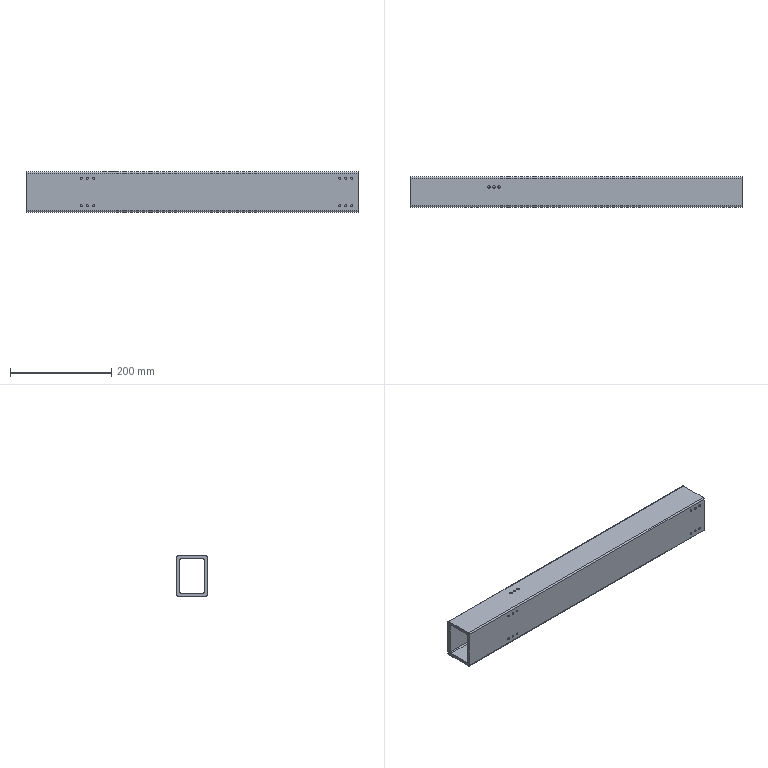Part | NX | 1 solid | 33 faces | box 656 x 60 x 80 mm | volume 1006265 mm3 | cylinder 23 | plane 10 | commonest cylinder face diameters 4.2 x12 5.236 x8 5 x3
STEP:
#1=CARTESIAN_POINT('',(30.,345.,37.382));
#2=VERTEX_POINT('',#1);
#3=CARTESIAN_POINT('',(30.,345.,-37.382));
#4=VERTEX_POINT('',#3);
#5=CARTESIAN_POINT('',(30.,345.,37.382));
#6=DIRECTION('',(0.,0.,-1.));
#7=VECTOR('',#6,1000.);
#8=LINE('',#5,#7);
#9=EDGE_CURVE('',#2,#4,#8,.T.);
#10=ORIENTED_EDGE('',*,*,#9,.F.);
#11=CARTESIAN_POINT('',(686.,345.,37.382));
#12=VERTEX_POINT('',#11);
#13=CARTESIAN_POINT('',(716.,345.,37.382));
#14=DIRECTION('',(-1.,0.,0.));
#15=VECTOR('',#14,1000.);
#16=LINE('',#13,#15);
#17=EDGE_CURVE('',#12,#2,#16,.T.);
#18=ORIENTED_EDGE('',*,*,#17,.F.);
#19=CARTESIAN_POINT('',(686.,345.,-37.382));
#20=VERTEX_POINT('',#19);
#21=CARTESIAN_POINT('',(686.,345.,37.382));
#22=DIRECTION('',(0.,0.,1.));
#23=VECTOR('',#22,1000.);
#24=LINE('',#21,#23);
#25=EDGE_CURVE('',#20,#12,#24,.T.);
#26=ORIENTED_EDGE('',*,*,#25,.F.);
#27=CARTESIAN_POINT('',(716.,345.,-37.382));
#28=DIRECTION('',(-1.,0.,0.));
#29=VECTOR('',#28,1000.);
#30=LINE('',#27,#29);
#31=EDGE_CURVE('',#20,#4,#30,.T.);
#32=ORIENTED_EDGE('',*,*,#31,.T.);
#33=EDGE_LOOP('',(#10,#18,#26,#32));
#34=FACE_BOUND('',#33,.T.);
#35=CARTESIAN_POINT('',(716.,345.,37.382));
#36=DIRECTION('',(0.,-1.,0.));
#37=DIRECTION('',(0.,0.,-1.));
#38=AXIS2_PLACEMENT_3D('',#35,#36,#37);
#39=PLANE('',#38);
#40=ADVANCED_FACE('',(#34),#39,.F.);
#41=CARTESIAN_POINT('',(30.,342.382,-40.));
#42=VERTEX_POINT('',#41);
#43=CARTESIAN_POINT('',(30.,342.382,-37.382));
#44=DIRECTION('',(-1.,0.,0.));
#45=DIRECTION('',(0.,0.,1.));
#46=AXIS2_PLACEMENT_3D('',#43,#44,#45);
#47=CIRCLE('',#46,2.618);
#48=EDGE_CURVE('',#4,#42,#47,.T.);
#49=ORIENTED_EDGE('',*,*,#48,.F.);
#50=ORIENTED_EDGE('',*,*,#31,.F.);
#51=CARTESIAN_POINT('',(686.,342.382,-40.));
#52=VERTEX_POINT('',#51);
#53=CARTESIAN_POINT('',(686.,342.382,-37.382));
#54=DIRECTION('',(1.,0.,0.));
#55=DIRECTION('',(0.,0.,-1.));
#56=AXIS2_PLACEMENT_3D('',#53,#54,#55);
#57=CIRCLE('',#56,2.618);
#58=EDGE_CURVE('',#52,#20,#57,.T.);
#59=ORIENTED_EDGE('',*,*,#58,.F.);
#60=CARTESIAN_POINT('',(716.,342.382,-40.));
#61=DIRECTION('',(-1.,0.,0.));
#62=VECTOR('',#61,1000.);
#63=LINE('',#60,#62);
#64=EDGE_CURVE('',#52,#42,#63,.T.);
#65=ORIENTED_EDGE('',*,*,#64,.T.);
#66=EDGE_LOOP('',(#49,#50,#59,#65));
#67=FACE_BOUND('',#66,.T.);
#68=CARTESIAN_POINT('',(716.,342.382,-37.382));
#69=DIRECTION('',(-1.,0.,0.));
#70=DIRECTION('',(0.,0.,1.));
#71=AXIS2_PLACEMENT_3D('',#68,#69,#70);
#72=CYLINDRICAL_SURFACE('',#71,2.618);
#73=ADVANCED_FACE('',(#67),#72,.T.);
#74=CARTESIAN_POINT('',(30.,287.618,-40.));
#75=VERTEX_POINT('',#74);
#76=CARTESIAN_POINT('',(30.,535.,-40.));
#77=DIRECTION('',(0.,-1.,0.));
#78=VECTOR('',#77,1000.);
#79=LINE('',#76,#78);
#80=EDGE_CURVE('',#42,#75,#79,.T.);
#81=ORIENTED_EDGE('',*,*,#80,.F.);
#82=ORIENTED_EDGE('',*,*,#64,.F.);
#83=CARTESIAN_POINT('',(686.,287.618,-40.));
#84=VERTEX_POINT('',#83);
#85=CARTESIAN_POINT('',(686.,535.,-40.));
#86=DIRECTION('',(0.,-1.,0.));
#87=VECTOR('',#86,1000.);
#88=LINE('',#85,#87);
#89=EDGE_CURVE('',#52,#84,#88,.T.);
#90=ORIENTED_EDGE('',*,*,#89,.T.);
#91=CARTESIAN_POINT('',(716.,287.618,-40.));
#92=DIRECTION('',(-1.,0.,0.));
#93=VECTOR('',#92,1000.);
#94=LINE('',#91,#93);
#95=EDGE_CURVE('',#84,#75,#94,.T.);
#96=ORIENTED_EDGE('',*,*,#95,.T.);
#97=EDGE_LOOP('',(#81,#82,#90,#96));
#98=FACE_BOUND('',#97,.T.);
#99=CARTESIAN_POINT('',(716.,287.618,-40.));
#100=DIRECTION('',(0.,0.,1.));
#101=DIRECTION('',(0.,-1.,0.));
#102=AXIS2_PLACEMENT_3D('',#99,#100,#101);
#103=PLANE('',#102);
#104=ADVANCED_FACE('',(#98),#103,.F.);
#105=CARTESIAN_POINT('',(30.,285.,-37.382));
#106=VERTEX_POINT('',#105);
#107=CARTESIAN_POINT('',(30.,287.618,-37.382));
#108=DIRECTION('',(-1.,0.,0.));
#109=DIRECTION('',(0.,0.,1.));
#110=AXIS2_PLACEMENT_3D('',#107,#108,#109);
#111=CIRCLE('',#110,2.618);
#112=EDGE_CURVE('',#75,#106,#111,.T.);
#113=ORIENTED_EDGE('',*,*,#112,.F.);
#114=ORIENTED_EDGE('',*,*,#95,.F.);
#115=CARTESIAN_POINT('',(686.,285.,-37.382));
#116=VERTEX_POINT('',#115);
#117=CARTESIAN_POINT('',(686.,287.618,-37.382));
#118=DIRECTION('',(1.,0.,0.));
#119=DIRECTION('',(0.,0.,-1.));
#120=AXIS2_PLACEMENT_3D('',#117,#118,#119);
#121=CIRCLE('',#120,2.618);
#122=EDGE_CURVE('',#116,#84,#121,.T.);
#123=ORIENTED_EDGE('',*,*,#122,.F.);
#124=CARTESIAN_POINT('',(716.,285.,-37.382));
#125=DIRECTION('',(-1.,0.,0.));
#126=VECTOR('',#125,1000.);
#127=LINE('',#124,#126);
#128=EDGE_CURVE('',#116,#106,#127,.T.);
#129=ORIENTED_EDGE('',*,*,#128,.T.);
#130=EDGE_LOOP('',(#113,#114,#123,#129));
#131=FACE_BOUND('',#130,.T.);
#132=CARTESIAN_POINT('',(716.,287.618,-37.382));
#133=DIRECTION('',(-1.,0.,0.));
#134=DIRECTION('',(0.,0.,1.));
#135=AXIS2_PLACEMENT_3D('',#132,#133,#134);
#136=CYLINDRICAL_SURFACE('',#135,2.618);
#137=ADVANCED_FACE('',(#131),#136,.T.);
#138=CARTESIAN_POINT('',(673.5,285.,25.4));
#139=VERTEX_POINT('',#138);
#140=CARTESIAN_POINT('',(673.5,285.,27.5));
#141=DIRECTION('',(0.,-1.,0.));
#142=DIRECTION('',(0.,0.,-1.));
#143=AXIS2_PLACEMENT_3D('',#140,#141,#142);
#144=CIRCLE('',#143,2.1);
#145=EDGE_CURVE('',#139,#139,#144,.T.);
#146=ORIENTED_EDGE('',*,*,#145,.F.);
#147=EDGE_LOOP('',(#146));
#148=FACE_BOUND('',#147,.T.);
#149=CARTESIAN_POINT('',(661.5,285.,25.4));
#150=VERTEX_POINT('',#149);
#151=CARTESIAN_POINT('',(661.5,285.,27.5));
#152=DIRECTION('',(0.,-1.,0.));
#153=DIRECTION('',(0.,0.,-1.));
#154=AXIS2_PLACEMENT_3D('',#151,#152,#153);
#155=CIRCLE('',#154,2.1);
#156=EDGE_CURVE('',#150,#150,#155,.T.);
#157=ORIENTED_EDGE('',*,*,#156,.F.);
#158=EDGE_LOOP('',(#157));
#159=FACE_BOUND('',#158,.T.);
#160=CARTESIAN_POINT('',(649.5,285.,25.4));
#161=VERTEX_POINT('',#160);
#162=CARTESIAN_POINT('',(649.5,285.,27.5));
#163=DIRECTION('',(0.,-1.,0.));
#164=DIRECTION('',(0.,0.,-1.));
#165=AXIS2_PLACEMENT_3D('',#162,#163,#164);
#166=CIRCLE('',#165,2.1);
#167=EDGE_CURVE('',#161,#161,#166,.T.);
#168=ORIENTED_EDGE('',*,*,#167,.F.);
#169=EDGE_LOOP('',(#168));
#170=FACE_BOUND('',#169,.T.);
#171=CARTESIAN_POINT('',(163.5,285.,25.4));
#172=VERTEX_POINT('',#171);
#173=CARTESIAN_POINT('',(163.5,285.,27.5));
#174=DIRECTION('',(0.,-1.,0.));
#175=DIRECTION('',(0.,0.,-1.));
#176=AXIS2_PLACEMENT_3D('',#173,#174,#175);
#177=CIRCLE('',#176,2.1);
#178=EDGE_CURVE('',#172,#172,#177,.T.);
#179=ORIENTED_EDGE('',*,*,#178,.F.);
#180=EDGE_LOOP('',(#179));
#181=FACE_BOUND('',#180,.T.);
#182=CARTESIAN_POINT('',(151.5,285.,25.4));
#183=VERTEX_POINT('',#182);
#184=CARTESIAN_POINT('',(151.5,285.,27.5));
#185=DIRECTION('',(0.,-1.,0.));
#186=DIRECTION('',(0.,0.,-1.));
#187=AXIS2_PLACEMENT_3D('',#184,#185,#186);
#188=CIRCLE('',#187,2.1);
#189=EDGE_CURVE('',#183,#183,#188,.T.);
#190=ORIENTED_EDGE('',*,*,#189,.F.);
#191=EDGE_LOOP('',(#190));
#192=FACE_BOUND('',#191,.T.);
#193=CARTESIAN_POINT('',(139.5,285.,25.4));
#194=VERTEX_POINT('',#193);
#195=CARTESIAN_POINT('',(139.5,285.,27.5));
#196=DIRECTION('',(0.,-1.,0.));
#197=DIRECTION('',(0.,0.,-1.));
#198=AXIS2_PLACEMENT_3D('',#195,#196,#197);
#199=CIRCLE('',#198,2.1);
#200=EDGE_CURVE('',#194,#194,#199,.T.);
#201=ORIENTED_EDGE('',*,*,#200,.F.);
#202=EDGE_LOOP('',(#201));
#203=FACE_BOUND('',#202,.T.);
#204=CARTESIAN_POINT('',(673.5,285.,-29.6));
#205=VERTEX_POINT('',#204);
#206=CARTESIAN_POINT('',(673.5,285.,-27.5));
#207=DIRECTION('',(0.,-1.,0.));
#208=DIRECTION('',(0.,0.,-1.));
#209=AXIS2_PLACEMENT_3D('',#206,#207,#208);
#210=CIRCLE('',#209,2.1);
#211=EDGE_CURVE('',#205,#205,#210,.T.);
#212=ORIENTED_EDGE('',*,*,#211,.F.);
#213=EDGE_LOOP('',(#212));
#214=FACE_BOUND('',#213,.T.);
#215=CARTESIAN_POINT('',(661.5,285.,-29.6));
#216=VERTEX_POINT('',#215);
#217=CARTESIAN_POINT('',(661.5,285.,-27.5));
#218=DIRECTION('',(0.,-1.,0.));
#219=DIRECTION('',(0.,0.,-1.));
#220=AXIS2_PLACEMENT_3D('',#217,#218,#219);
#221=CIRCLE('',#220,2.1);
#222=EDGE_CURVE('',#216,#216,#221,.T.);
#223=ORIENTED_EDGE('',*,*,#222,.F.);
#224=EDGE_LOOP('',(#223));
#225=FACE_BOUND('',#224,.T.);
#226=CARTESIAN_POINT('',(649.5,285.,-29.6));
#227=VERTEX_POINT('',#226);
#228=CARTESIAN_POINT('',(649.5,285.,-27.5));
#229=DIRECTION('',(0.,-1.,0.));
#230=DIRECTION('',(0.,0.,-1.));
#231=AXIS2_PLACEMENT_3D('',#228,#229,#230);
#232=CIRCLE('',#231,2.1);
#233=EDGE_CURVE('',#227,#227,#232,.T.);
#234=ORIENTED_EDGE('',*,*,#233,.F.);
#235=EDGE_LOOP('',(#234));
#236=FACE_BOUND('',#235,.T.);
#237=CARTESIAN_POINT('',(163.5,285.,-29.6));
#238=VERTEX_POINT('',#237);
#239=CARTESIAN_POINT('',(163.5,285.,-27.5));
#240=DIRECTION('',(0.,-1.,0.));
#241=DIRECTION('',(0.,0.,-1.));
#242=AXIS2_PLACEMENT_3D('',#239,#240,#241);
#243=CIRCLE('',#242,2.1);
#244=EDGE_CURVE('',#238,#238,#243,.T.);
#245=ORIENTED_EDGE('',*,*,#244,.F.);
#246=EDGE_LOOP('',(#245));
#247=FACE_BOUND('',#246,.T.);
#248=CARTESIAN_POINT('',(151.5,285.,-29.6));
#249=VERTEX_POINT('',#248);
#250=CARTESIAN_POINT('',(151.5,285.,-27.5));
#251=DIRECTION('',(0.,-1.,0.));
#252=DIRECTION('',(0.,0.,-1.));
#253=AXIS2_PLACEMENT_3D('',#250,#251,#252);
#254=CIRCLE('',#253,2.1);
#255=EDGE_CURVE('',#249,#249,#254,.T.);
#256=ORIENTED_EDGE('',*,*,#255,.F.);
#257=EDGE_LOOP('',(#256));
#258=FACE_BOUND('',#257,.T.);
#259=CARTESIAN_POINT('',(139.5,285.,-29.6));
#260=VERTEX_POINT('',#259);
#261=CARTESIAN_POINT('',(139.5,285.,-27.5));
#262=DIRECTION('',(0.,-1.,0.));
#263=DIRECTION('',(0.,0.,-1.));
#264=AXIS2_PLACEMENT_3D('',#261,#262,#263);
#265=CIRCLE('',#264,2.1);
#266=EDGE_CURVE('',#260,#260,#265,.T.);
#267=ORIENTED_EDGE('',*,*,#266,.F.);
#268=EDGE_LOOP('',(#267));
#269=FACE_BOUND('',#268,.T.);
#270=CARTESIAN_POINT('',(30.,285.,37.382));
#271=VERTEX_POINT('',#270);
#272=CARTESIAN_POINT('',(30.,285.,37.382));
#273=DIRECTION('',(0.,0.,1.));
#274=VECTOR('',#273,1000.);
#275=LINE('',#272,#274);
#276=EDGE_CURVE('',#106,#271,#275,.T.);
#277=ORIENTED_EDGE('',*,*,#276,.F.);
#278=ORIENTED_EDGE('',*,*,#128,.F.);
#279=CARTESIAN_POINT('',(686.,285.,37.382));
#280=VERTEX_POINT('',#279);
#281=CARTESIAN_POINT('',(686.,285.,37.382));
#282=DIRECTION('',(0.,0.,-1.));
#283=VECTOR('',#282,1000.);
#284=LINE('',#281,#283);
#285=EDGE_CURVE('',#280,#116,#284,.T.);
#286=ORIENTED_EDGE('',*,*,#285,.F.);
#287=CARTESIAN_POINT('',(716.,285.,37.382));
#288=DIRECTION('',(-1.,0.,0.));
#289=VECTOR('',#288,1000.);
#290=LINE('',#287,#289);
#291=EDGE_CURVE('',#280,#271,#290,.T.);
#292=ORIENTED_EDGE('',*,*,#291,.T.);
#293=EDGE_LOOP('',(#277,#278,#286,#292));
#294=FACE_BOUND('',#293,.T.);
#295=CARTESIAN_POINT('',(716.,285.,37.382));
#296=DIRECTION('',(0.,1.,0.));
#297=DIRECTION('',(0.,0.,1.));
#298=AXIS2_PLACEMENT_3D('',#295,#296,#297);
#299=PLANE('',#298);
#300=ADVANCED_FACE('',(#148,#159,#170,#181,#192,#203,#214,#225,#236,#247,#258,#269,#294),#299,.F.);
#301=CARTESIAN_POINT('',(30.,287.618,40.));
#302=VERTEX_POINT('',#301);
#303=CARTESIAN_POINT('',(30.,287.618,37.382));
#304=DIRECTION('',(-1.,0.,0.));
#305=DIRECTION('',(0.,0.,1.));
#306=AXIS2_PLACEMENT_3D('',#303,#304,#305);
#307=CIRCLE('',#306,2.618);
#308=EDGE_CURVE('',#271,#302,#307,.T.);
#309=ORIENTED_EDGE('',*,*,#308,.F.);
#310=ORIENTED_EDGE('',*,*,#291,.F.);
#311=CARTESIAN_POINT('',(686.,287.618,40.));
#312=VERTEX_POINT('',#311);
#313=CARTESIAN_POINT('',(686.,287.618,37.382));
#314=DIRECTION('',(1.,0.,0.));
#315=DIRECTION('',(0.,0.,-1.));
#316=AXIS2_PLACEMENT_3D('',#313,#314,#315);
#317=CIRCLE('',#316,2.618);
#318=EDGE_CURVE('',#312,#280,#317,.T.);
#319=ORIENTED_EDGE('',*,*,#318,.F.);
#320=CARTESIAN_POINT('',(716.,287.618,40.));
#321=DIRECTION('',(-1.,0.,0.));
#322=VECTOR('',#321,1000.);
#323=LINE('',#320,#322);
#324=EDGE_CURVE('',#312,#302,#323,.T.);
#325=ORIENTED_EDGE('',*,*,#324,.T.);
#326=EDGE_LOOP('',(#309,#310,#319,#325));
#327=FACE_BOUND('',#326,.T.);
#328=CARTESIAN_POINT('',(716.,287.618,37.382));
#329=DIRECTION('',(-1.,0.,0.));
#330=DIRECTION('',(0.,0.,1.));
#331=AXIS2_PLACEMENT_3D('',#328,#329,#330);
#332=CYLINDRICAL_SURFACE('',#331,2.618);
#333=ADVANCED_FACE('',(#327),#332,.T.);
#334=CARTESIAN_POINT('',(206.,322.5,40.));
#335=VERTEX_POINT('',#334);
#336=CARTESIAN_POINT('',(206.,325.,40.));
#337=DIRECTION('',(0.,0.,1.));
#338=DIRECTION('',(0.,-1.,0.));
#339=AXIS2_PLACEMENT_3D('',#336,#337,#338);
#340=CIRCLE('',#339,2.5);
#341=EDGE_CURVE('',#335,#335,#340,.T.);
#342=ORIENTED_EDGE('',*,*,#341,.F.);
#343=EDGE_LOOP('',(#342));
#344=FACE_BOUND('',#343,.T.);
#345=CARTESIAN_POINT('',(186.,322.5,40.));
#346=VERTEX_POINT('',#345);
#347=CARTESIAN_POINT('',(186.,325.,40.));
#348=DIRECTION('',(0.,0.,1.));
#349=DIRECTION('',(0.,-1.,0.));
#350=AXIS2_PLACEMENT_3D('',#347,#348,#349);
#351=CIRCLE('',#350,2.5);
#352=EDGE_CURVE('',#346,#346,#351,.T.);
#353=ORIENTED_EDGE('',*,*,#352,.F.);
#354=EDGE_LOOP('',(#353));
#355=FACE_BOUND('',#354,.T.);
#356=CARTESIAN_POINT('',(196.,322.5,40.));
#357=VERTEX_POINT('',#356);
#358=CARTESIAN_POINT('',(196.,325.,40.));
#359=DIRECTION('',(0.,0.,1.));
#360=DIRECTION('',(0.,-1.,0.));
#361=AXIS2_PLACEMENT_3D('',#358,#359,#360);
#362=CIRCLE('',#361,2.5);
#363=EDGE_CURVE('',#357,#357,#362,.T.);
#364=ORIENTED_EDGE('',*,*,#363,.F.);
#365=EDGE_LOOP('',(#364));
#366=FACE_BOUND('',#365,.T.);
#367=CARTESIAN_POINT('',(30.,342.382,40.));
#368=VERTEX_POINT('',#367);
#369=CARTESIAN_POINT('',(30.,535.,40.));
#370=DIRECTION('',(0.,-1.,0.));
#371=VECTOR('',#370,1000.);
#372=LINE('',#369,#371);
#373=EDGE_CURVE('',#368,#302,#372,.T.);
#374=ORIENTED_EDGE('',*,*,#373,.T.);
#375=ORIENTED_EDGE('',*,*,#324,.F.);
#376=CARTESIAN_POINT('',(686.,342.382,40.));
#377=VERTEX_POINT('',#376);
#378=CARTESIAN_POINT('',(686.,535.,40.));
#379=DIRECTION('',(0.,-1.,0.));
#380=VECTOR('',#379,1000.);
#381=LINE('',#378,#380);
#382=EDGE_CURVE('',#377,#312,#381,.T.);
#383=ORIENTED_EDGE('',*,*,#382,.F.);
#384=CARTESIAN_POINT('',(716.,342.382,40.));
#385=DIRECTION('',(-1.,0.,0.));
#386=VECTOR('',#385,1000.);
#387=LINE('',#384,#386);
#388=EDGE_CURVE('',#377,#368,#387,.T.);
#389=ORIENTED_EDGE('',*,*,#388,.T.);
#390=EDGE_LOOP('',(#374,#375,#383,#389));
#391=FACE_BOUND('',#390,.T.);
#392=CARTESIAN_POINT('',(716.,287.618,40.));
#393=DIRECTION('',(0.,0.,-1.));
#394=DIRECTION('',(0.,1.,0.));
#395=AXIS2_PLACEMENT_3D('',#392,#393,#394);
#396=PLANE('',#395);
#397=ADVANCED_FACE('',(#344,#355,#366,#391),#396,.F.);
#398=CARTESIAN_POINT('',(30.,342.382,37.382));
#399=DIRECTION('',(-1.,0.,0.));
#400=DIRECTION('',(0.,0.,1.));
#401=AXIS2_PLACEMENT_3D('',#398,#399,#400);
#402=CIRCLE('',#401,2.618);
#403=EDGE_CURVE('',#368,#2,#402,.T.);
#404=ORIENTED_EDGE('',*,*,#403,.F.);
#405=ORIENTED_EDGE('',*,*,#388,.F.);
#406=CARTESIAN_POINT('',(686.,342.382,37.382));
#407=DIRECTION('',(1.,0.,0.));
#408=DIRECTION('',(0.,0.,-1.));
#409=AXIS2_PLACEMENT_3D('',#406,#407,#408);
#410=CIRCLE('',#409,2.618);
#411=EDGE_CURVE('',#12,#377,#410,.T.);
#412=ORIENTED_EDGE('',*,*,#411,.F.);
#413=ORIENTED_EDGE('',*,*,#17,.T.);
#414=EDGE_LOOP('',(#404,#405,#412,#413));
#415=FACE_BOUND('',#414,.T.);
#416=CARTESIAN_POINT('',(716.,342.382,37.382));
#417=DIRECTION('',(-1.,0.,0.));
#418=DIRECTION('',(0.,0.,1.));
#419=AXIS2_PLACEMENT_3D('',#416,#417,#418);
#420=CYLINDRICAL_SURFACE('',#419,2.618);
#421=ADVANCED_FACE('',(#415),#420,.T.);
#422=CARTESIAN_POINT('',(686.,336.382,-34.));
#423=VERTEX_POINT('',#422);
#424=CARTESIAN_POINT('',(30.,336.382,-34.));
#425=VERTEX_POINT('',#424);
#426=CARTESIAN_POINT('',(716.,336.382,-34.));
#427=DIRECTION('',(-1.,0.,0.));
#428=VECTOR('',#427,1000.);
#429=LINE('',#426,#428);
#430=EDGE_CURVE('',#423,#425,#429,.T.);
#431=ORIENTED_EDGE('',*,*,#430,.T.);
#432=CARTESIAN_POINT('',(30.,293.618,-34.));
#433=VERTEX_POINT('',#432);
#434=CARTESIAN_POINT('',(30.,293.618,-34.));
#435=DIRECTION('',(0.,-1.,0.));
#436=VECTOR('',#435,1000.);
#437=LINE('',#434,#436);
#438=EDGE_CURVE('',#425,#433,#437,.T.);
#439=ORIENTED_EDGE('',*,*,#438,.T.);
#440=CARTESIAN_POINT('',(686.,293.618,-34.));
#441=VERTEX_POINT('',#440);
#442=CARTESIAN_POINT('',(716.,293.618,-34.));
#443=DIRECTION('',(-1.,0.,0.));
#444=VECTOR('',#443,1000.);
#445=LINE('',#442,#444);
#446=EDGE_CURVE('',#441,#433,#445,.T.);
#447=ORIENTED_EDGE('',*,*,#446,.F.);
#448=CARTESIAN_POINT('',(686.,293.618,-34.));
#449=DIRECTION('',(0.,1.,0.));
#450=VECTOR('',#449,1000.);
#451=LINE('',#448,#450);
#452=EDGE_CURVE('',#441,#423,#451,.T.);
#453=ORIENTED_EDGE('',*,*,#452,.T.);
#454=EDGE_LOOP('',(#431,#439,#447,#453));
#455=FACE_BOUND('',#454,.T.);
#456=CARTESIAN_POINT('',(716.,293.618,-34.));
#457=DIRECTION('',(0.,0.,1.));
#458=DIRECTION('',(0.,-1.,0.));
#459=AXIS2_PLACEMENT_3D('',#456,#457,#458);
#460=PLANE('',#459);
#461=ADVANCED_FACE('',(#455),#460,.T.);
#462=CARTESIAN_POINT('',(686.,339.,-31.382));
#463=VERTEX_POINT('',#462);
#464=CARTESIAN_POINT('',(30.,339.,-31.382));
#465=VERTEX_POINT('',#464);
#466=CARTESIAN_POINT('',(716.,339.,-31.382));
#467=DIRECTION('',(-1.,0.,0.));
#468=VECTOR('',#467,1000.);
#469=LINE('',#466,#468);
#470=EDGE_CURVE('',#463,#465,#469,.T.);
#471=ORIENTED_EDGE('',*,*,#470,.T.);
#472=CARTESIAN_POINT('',(30.,336.382,-31.382));
#473=DIRECTION('',(-1.,0.,0.));
#474=DIRECTION('',(0.,0.,1.));
#475=AXIS2_PLACEMENT_3D('',#472,#473,#474);
#476=CIRCLE('',#475,2.618);
#477=EDGE_CURVE('',#465,#425,#476,.T.);
#478=ORIENTED_EDGE('',*,*,#477,.T.);
#479=ORIENTED_EDGE('',*,*,#430,.F.);
#480=CARTESIAN_POINT('',(686.,336.382,-31.382));
#481=DIRECTION('',(1.,0.,0.));
#482=DIRECTION('',(0.,0.,-1.));
#483=AXIS2_PLACEMENT_3D('',#480,#481,#482);
#484=CIRCLE('',#483,2.618);
#485=EDGE_CURVE('',#423,#463,#484,.T.);
#486=ORIENTED_EDGE('',*,*,#485,.T.);
#487=EDGE_LOOP('',(#471,#478,#479,#486));
#488=FACE_BOUND('',#487,.T.);
#489=CARTESIAN_POINT('',(716.,336.382,-31.382));
#490=DIRECTION('',(-1.,0.,0.));
#491=DIRECTION('',(0.,0.,1.));
#492=AXIS2_PLACEMENT_3D('',#489,#490,#491);
#493=CYLINDRICAL_SURFACE('',#492,2.618);
#494=ADVANCED_FACE('',(#488),#493,.F.);
#495=CARTESIAN_POINT('',(686.,339.,31.382));
#496=VERTEX_POINT('',#495);
#497=CARTESIAN_POINT('',(30.,339.,31.382));
#498=VERTEX_POINT('',#497);
#499=CARTESIAN_POINT('',(716.,339.,31.382));
#500=DIRECTION('',(-1.,0.,0.));
#501=VECTOR('',#500,1000.);
#502=LINE('',#499,#501);
#503=EDGE_CURVE('',#496,#498,#502,.T.);
#504=ORIENTED_EDGE('',*,*,#503,.T.);
#505=CARTESIAN_POINT('',(30.,339.,31.382));
#506=DIRECTION('',(0.,0.,-1.));
#507=VECTOR('',#506,1000.);
#508=LINE('',#505,#507);
#509=EDGE_CURVE('',#498,#465,#508,.T.);
#510=ORIENTED_EDGE('',*,*,#509,.T.);
#511=ORIENTED_EDGE('',*,*,#470,.F.);
#512=CARTESIAN_POINT('',(686.,339.,31.382));
#513=DIRECTION('',(0.,0.,1.));
#514=VECTOR('',#513,1000.);
#515=LINE('',#512,#514);
#516=EDGE_CURVE('',#463,#496,#515,.T.);
#517=ORIENTED_EDGE('',*,*,#516,.T.);
#518=EDGE_LOOP('',(#504,#510,#511,#517));
#519=FACE_BOUND('',#518,.T.);
#520=CARTESIAN_POINT('',(716.,339.,31.382));
#521=DIRECTION('',(0.,-1.,0.));
#522=DIRECTION('',(0.,0.,-1.));
#523=AXIS2_PLACEMENT_3D('',#520,#521,#522);
#524=PLANE('',#523);
#525=ADVANCED_FACE('',(#519),#524,.T.);
#526=CARTESIAN_POINT('',(686.,336.382,34.));
#527=VERTEX_POINT('',#526);
#528=CARTESIAN_POINT('',(30.,336.382,34.));
#529=VERTEX_POINT('',#528);
#530=CARTESIAN_POINT('',(716.,336.382,34.));
#531=DIRECTION('',(-1.,0.,0.));
#532=VECTOR('',#531,1000.);
#533=LINE('',#530,#532);
#534=EDGE_CURVE('',#527,#529,#533,.T.);
#535=ORIENTED_EDGE('',*,*,#534,.T.);
#536=CARTESIAN_POINT('',(30.,336.382,31.382));
#537=DIRECTION('',(-1.,0.,0.));
#538=DIRECTION('',(0.,0.,1.));
#539=AXIS2_PLACEMENT_3D('',#536,#537,#538);
#540=CIRCLE('',#539,2.618);
#541=EDGE_CURVE('',#529,#498,#540,.T.);
#542=ORIENTED_EDGE('',*,*,#541,.T.);
#543=ORIENTED_EDGE('',*,*,#503,.F.);
#544=CARTESIAN_POINT('',(686.,336.382,31.382));
#545=DIRECTION('',(1.,0.,0.));
#546=DIRECTION('',(0.,0.,-1.));
#547=AXIS2_PLACEMENT_3D('',#544,#545,#546);
#548=CIRCLE('',#547,2.618);
#549=EDGE_CURVE('',#496,#527,#548,.T.);
#550=ORIENTED_EDGE('',*,*,#549,.T.);
#551=EDGE_LOOP('',(#535,#542,#543,#550));
#552=FACE_BOUND('',#551,.T.);
#553=CARTESIAN_POINT('',(716.,336.382,31.382));
#554=DIRECTION('',(-1.,0.,0.));
#555=DIRECTION('',(0.,0.,1.));
#556=AXIS2_PLACEMENT_3D('',#553,#554,#555);
#557=CYLINDRICAL_SURFACE('',#556,2.618);
#558=ADVANCED_FACE('',(#552),#557,.F.);
#559=CARTESIAN_POINT('',(206.,327.5,34.));
#560=VERTEX_POINT('',#559);
#561=CARTESIAN_POINT('',(206.,325.,34.));
#562=DIRECTION('',(0.,0.,-1.));
#563=DIRECTION('',(0.,1.,0.));
#564=AXIS2_PLACEMENT_3D('',#561,#562,#563);
#565=CIRCLE('',#564,2.5);
#566=EDGE_CURVE('',#560,#560,#565,.T.);
#567=ORIENTED_EDGE('',*,*,#566,.F.);
#568=EDGE_LOOP('',(#567));
#569=FACE_BOUND('',#568,.T.);
#570=CARTESIAN_POINT('',(186.,327.5,34.));
#571=VERTEX_POINT('',#570);
#572=CARTESIAN_POINT('',(186.,325.,34.));
#573=DIRECTION('',(0.,0.,-1.));
#574=DIRECTION('',(0.,1.,0.));
#575=AXIS2_PLACEMENT_3D('',#572,#573,#574);
#576=CIRCLE('',#575,2.5);
#577=EDGE_CURVE('',#571,#571,#576,.T.);
#578=ORIENTED_EDGE('',*,*,#577,.F.);
#579=EDGE_LOOP('',(#578));
#580=FACE_BOUND('',#579,.T.);
#581=CARTESIAN_POINT('',(196.,327.5,34.));
#582=VERTEX_POINT('',#581);
#583=CARTESIAN_POINT('',(196.,325.,34.));
#584=DIRECTION('',(0.,0.,-1.));
#585=DIRECTION('',(0.,1.,0.));
#586=AXIS2_PLACEMENT_3D('',#583,#584,#585);
#587=CIRCLE('',#586,2.5);
#588=EDGE_CURVE('',#582,#582,#587,.T.);
#589=ORIENTED_EDGE('',*,*,#588,.F.);
#590=EDGE_LOOP('',(#589));
#591=FACE_BOUND('',#590,.T.);
#592=CARTESIAN_POINT('',(686.,293.618,34.));
#593=VERTEX_POINT('',#592);
#594=CARTESIAN_POINT('',(30.,293.618,34.));
#595=VERTEX_POINT('',#594);
#596=CARTESIAN_POINT('',(716.,293.618,34.));
#597=DIRECTION('',(-1.,0.,0.));
#598=VECTOR('',#597,1000.);
#599=LINE('',#596,#598);
#600=EDGE_CURVE('',#593,#595,#599,.T.);
#601=ORIENTED_EDGE('',*,*,#600,.T.);
#602=CARTESIAN_POINT('',(30.,293.618,34.));
#603=DIRECTION('',(0.,1.,0.));
#604=VECTOR('',#603,1000.);
#605=LINE('',#602,#604);
#606=EDGE_CURVE('',#595,#529,#605,.T.);
#607=ORIENTED_EDGE('',*,*,#606,.T.);
#608=ORIENTED_EDGE('',*,*,#534,.F.);
#609=CARTESIAN_POINT('',(686.,293.618,34.));
#610=DIRECTION('',(0.,-1.,0.));
#611=VECTOR('',#610,1000.);
#612=LINE('',#609,#611);
#613=EDGE_CURVE('',#527,#593,#612,.T.);
#614=ORIENTED_EDGE('',*,*,#613,.T.);
#615=EDGE_LOOP('',(#601,#607,#608,#614));
#616=FACE_BOUND('',#615,.T.);
#617=CARTESIAN_POINT('',(716.,293.618,34.));
#618=DIRECTION('',(0.,0.,-1.));
#619=DIRECTION('',(0.,1.,0.));
#620=AXIS2_PLACEMENT_3D('',#617,#618,#619);
#621=PLANE('',#620);
#622=ADVANCED_FACE('',(#569,#580,#591,#616),#621,.T.);
#623=CARTESIAN_POINT('',(686.,291.,31.382));
#624=VERTEX_POINT('',#623);
#625=CARTESIAN_POINT('',(30.,291.,31.382));
#626=VERTEX_POINT('',#625);
#627=CARTESIAN_POINT('',(716.,291.,31.382));
#628=DIRECTION('',(-1.,0.,0.));
#629=VECTOR('',#628,1000.);
#630=LINE('',#627,#629);
#631=EDGE_CURVE('',#624,#626,#630,.T.);
#632=ORIENTED_EDGE('',*,*,#631,.T.);
#633=CARTESIAN_POINT('',(30.,293.618,31.382));
#634=DIRECTION('',(-1.,0.,0.));
#635=DIRECTION('',(0.,0.,1.));
#636=AXIS2_PLACEMENT_3D('',#633,#634,#635);
#637=CIRCLE('',#636,2.618);
#638=EDGE_CURVE('',#626,#595,#637,.T.);
#639=ORIENTED_EDGE('',*,*,#638,.T.);
#640=ORIENTED_EDGE('',*,*,#600,.F.);
#641=CARTESIAN_POINT('',(686.,293.618,31.382));
#642=DIRECTION('',(1.,0.,0.));
#643=DIRECTION('',(0.,0.,-1.));
#644=AXIS2_PLACEMENT_3D('',#641,#642,#643);
#645=CIRCLE('',#644,2.618);
#646=EDGE_CURVE('',#593,#624,#645,.T.);
#647=ORIENTED_EDGE('',*,*,#646,.T.);
#648=EDGE_LOOP('',(#632,#639,#640,#647));
#649=FACE_BOUND('',#648,.T.);
#650=CARTESIAN_POINT('',(716.,293.618,31.382));
#651=DIRECTION('',(-1.,0.,0.));
#652=DIRECTION('',(0.,0.,1.));
#653=AXIS2_PLACEMENT_3D('',#650,#651,#652);
#654=CYLINDRICAL_SURFACE('',#653,2.618);
#655=ADVANCED_FACE('',(#649),#654,.F.);
#656=CARTESIAN_POINT('',(673.5,291.,29.6));
#657=VERTEX_POINT('',#656);
#658=CARTESIAN_POINT('',(673.5,291.,27.5));
#659=DIRECTION('',(0.,1.,0.));
#660=DIRECTION('',(0.,0.,1.));
#661=AXIS2_PLACEMENT_3D('',#658,#659,#660);
#662=CIRCLE('',#661,2.1);
#663=EDGE_CURVE('',#657,#657,#662,.T.);
#664=ORIENTED_EDGE('',*,*,#663,.F.);
#665=EDGE_LOOP('',(#664));
#666=FACE_BOUND('',#665,.T.);
#667=CARTESIAN_POINT('',(661.5,291.,29.6));
#668=VERTEX_POINT('',#667);
#669=CARTESIAN_POINT('',(661.5,291.,27.5));
#670=DIRECTION('',(0.,1.,0.));
#671=DIRECTION('',(0.,0.,1.));
#672=AXIS2_PLACEMENT_3D('',#669,#670,#671);
#673=CIRCLE('',#672,2.1);
#674=EDGE_CURVE('',#668,#668,#673,.T.);
#675=ORIENTED_EDGE('',*,*,#674,.F.);
#676=EDGE_LOOP('',(#675));
#677=FACE_BOUND('',#676,.T.);
#678=CARTESIAN_POINT('',(649.5,291.,29.6));
#679=VERTEX_POINT('',#678);
#680=CARTESIAN_POINT('',(649.5,291.,27.5));
#681=DIRECTION('',(0.,1.,0.));
#682=DIRECTION('',(0.,0.,1.));
#683=AXIS2_PLACEMENT_3D('',#680,#681,#682);
#684=CIRCLE('',#683,2.1);
#685=EDGE_CURVE('',#679,#679,#684,.T.);
#686=ORIENTED_EDGE('',*,*,#685,.F.);
#687=EDGE_LOOP('',(#686));
#688=FACE_BOUND('',#687,.T.);
#689=CARTESIAN_POINT('',(163.5,291.,29.6));
#690=VERTEX_POINT('',#689);
#691=CARTESIAN_POINT('',(163.5,291.,27.5));
#692=DIRECTION('',(0.,1.,0.));
#693=DIRECTION('',(0.,0.,1.));
#694=AXIS2_PLACEMENT_3D('',#691,#692,#693);
#695=CIRCLE('',#694,2.1);
#696=EDGE_CURVE('',#690,#690,#695,.T.);
#697=ORIENTED_EDGE('',*,*,#696,.F.);
#698=EDGE_LOOP('',(#697));
#699=FACE_BOUND('',#698,.T.);
#700=CARTESIAN_POINT('',(151.5,291.,29.6));
#701=VERTEX_POINT('',#700);
#702=CARTESIAN_POINT('',(151.5,291.,27.5));
#703=DIRECTION('',(0.,1.,0.));
#704=DIRECTION('',(0.,0.,1.));
#705=AXIS2_PLACEMENT_3D('',#702,#703,#704);
#706=CIRCLE('',#705,2.1);
#707=EDGE_CURVE('',#701,#701,#706,.T.);
#708=ORIENTED_EDGE('',*,*,#707,.F.);
#709=EDGE_LOOP('',(#708));
#710=FACE_BOUND('',#709,.T.);
#711=CARTESIAN_POINT('',(139.5,291.,29.6));
#712=VERTEX_POINT('',#711);
#713=CARTESIAN_POINT('',(139.5,291.,27.5));
#714=DIRECTION('',(0.,1.,0.));
#715=DIRECTION('',(0.,0.,1.));
#716=AXIS2_PLACEMENT_3D('',#713,#714,#715);
#717=CIRCLE('',#716,2.1);
#718=EDGE_CURVE('',#712,#712,#717,.T.);
#719=ORIENTED_EDGE('',*,*,#718,.F.);
#720=EDGE_LOOP('',(#719));
#721=FACE_BOUND('',#720,.T.);
#722=CARTESIAN_POINT('',(673.5,291.,-25.4));
#723=VERTEX_POINT('',#722);
#724=CARTESIAN_POINT('',(673.5,291.,-27.5));
#725=DIRECTION('',(0.,1.,0.));
#726=DIRECTION('',(0.,0.,1.));
#727=AXIS2_PLACEMENT_3D('',#724,#725,#726);
#728=CIRCLE('',#727,2.1);
#729=EDGE_CURVE('',#723,#723,#728,.T.);
#730=ORIENTED_EDGE('',*,*,#729,.F.);
#731=EDGE_LOOP('',(#730));
#732=FACE_BOUND('',#731,.T.);
#733=CARTESIAN_POINT('',(661.5,291.,-25.4));
#734=VERTEX_POINT('',#733);
#735=CARTESIAN_POINT('',(661.5,291.,-27.5));
#736=DIRECTION('',(0.,1.,0.));
#737=DIRECTION('',(0.,0.,1.));
#738=AXIS2_PLACEMENT_3D('',#735,#736,#737);
#739=CIRCLE('',#738,2.1);
#740=EDGE_CURVE('',#734,#734,#739,.T.);
#741=ORIENTED_EDGE('',*,*,#740,.F.);
#742=EDGE_LOOP('',(#741));
#743=FACE_BOUND('',#742,.T.);
#744=CARTESIAN_POINT('',(649.5,291.,-25.4));
#745=VERTEX_POINT('',#744);
#746=CARTESIAN_POINT('',(649.5,291.,-27.5));
#747=DIRECTION('',(0.,1.,0.));
#748=DIRECTION('',(0.,0.,1.));
#749=AXIS2_PLACEMENT_3D('',#746,#747,#748);
#750=CIRCLE('',#749,2.1);
#751=EDGE_CURVE('',#745,#745,#750,.T.);
#752=ORIENTED_EDGE('',*,*,#751,.F.);
#753=EDGE_LOOP('',(#752));
#754=FACE_BOUND('',#753,.T.);
#755=CARTESIAN_POINT('',(163.5,291.,-25.4));
#756=VERTEX_POINT('',#755);
#757=CARTESIAN_POINT('',(163.5,291.,-27.5));
#758=DIRECTION('',(0.,1.,0.));
#759=DIRECTION('',(0.,0.,1.));
#760=AXIS2_PLACEMENT_3D('',#757,#758,#759);
#761=CIRCLE('',#760,2.1);
#762=EDGE_CURVE('',#756,#756,#761,.T.);
#763=ORIENTED_EDGE('',*,*,#762,.F.);
#764=EDGE_LOOP('',(#763));
#765=FACE_BOUND('',#764,.T.);
#766=CARTESIAN_POINT('',(151.5,291.,-25.4));
#767=VERTEX_POINT('',#766);
#768=CARTESIAN_POINT('',(151.5,291.,-27.5));
#769=DIRECTION('',(0.,1.,0.));
#770=DIRECTION('',(0.,0.,1.));
#771=AXIS2_PLACEMENT_3D('',#768,#769,#770);
#772=CIRCLE('',#771,2.1);
#773=EDGE_CURVE('',#767,#767,#772,.T.);
#774=ORIENTED_EDGE('',*,*,#773,.F.);
#775=EDGE_LOOP('',(#774));
#776=FACE_BOUND('',#775,.T.);
#777=CARTESIAN_POINT('',(139.5,291.,-25.4));
#778=VERTEX_POINT('',#777);
#779=CARTESIAN_POINT('',(139.5,291.,-27.5));
#780=DIRECTION('',(0.,1.,0.));
#781=DIRECTION('',(0.,0.,1.));
#782=AXIS2_PLACEMENT_3D('',#779,#780,#781);
#783=CIRCLE('',#782,2.1);
#784=EDGE_CURVE('',#778,#778,#783,.T.);
#785=ORIENTED_EDGE('',*,*,#784,.F.);
#786=EDGE_LOOP('',(#785));
#787=FACE_BOUND('',#786,.T.);
#788=CARTESIAN_POINT('',(686.,291.,-31.382));
#789=VERTEX_POINT('',#788);
#790=CARTESIAN_POINT('',(30.,291.,-31.382));
#791=VERTEX_POINT('',#790);
#792=CARTESIAN_POINT('',(716.,291.,-31.382));
#793=DIRECTION('',(-1.,0.,0.));
#794=VECTOR('',#793,1000.);
#795=LINE('',#792,#794);
#796=EDGE_CURVE('',#789,#791,#795,.T.);
#797=ORIENTED_EDGE('',*,*,#796,.T.);
#798=CARTESIAN_POINT('',(30.,291.,31.382));
#799=DIRECTION('',(0.,0.,1.));
#800=VECTOR('',#799,1000.);
#801=LINE('',#798,#800);
#802=EDGE_CURVE('',#791,#626,#801,.T.);
#803=ORIENTED_EDGE('',*,*,#802,.T.);
#804=ORIENTED_EDGE('',*,*,#631,.F.);
#805=CARTESIAN_POINT('',(686.,291.,31.382));
#806=DIRECTION('',(0.,0.,-1.));
#807=VECTOR('',#806,1000.);
#808=LINE('',#805,#807);
#809=EDGE_CURVE('',#624,#789,#808,.T.);
#810=ORIENTED_EDGE('',*,*,#809,.T.);
#811=EDGE_LOOP('',(#797,#803,#804,#810));
#812=FACE_BOUND('',#811,.T.);
#813=CARTESIAN_POINT('',(716.,291.,31.382));
#814=DIRECTION('',(0.,1.,0.));
#815=DIRECTION('',(0.,0.,1.));
#816=AXIS2_PLACEMENT_3D('',#813,#814,#815);
#817=PLANE('',#816);
#818=ADVANCED_FACE('',(#666,#677,#688,#699,#710,#721,#732,#743,#754,#765,#776,#787,#812),#817,.T.);
#819=ORIENTED_EDGE('',*,*,#446,.T.);
#820=CARTESIAN_POINT('',(30.,293.618,-31.382));
#821=DIRECTION('',(-1.,0.,0.));
#822=DIRECTION('',(0.,0.,1.));
#823=AXIS2_PLACEMENT_3D('',#820,#821,#822);
#824=CIRCLE('',#823,2.618);
#825=EDGE_CURVE('',#433,#791,#824,.T.);
#826=ORIENTED_EDGE('',*,*,#825,.T.);
#827=ORIENTED_EDGE('',*,*,#796,.F.);
#828=CARTESIAN_POINT('',(686.,293.618,-31.382));
#829=DIRECTION('',(1.,0.,0.));
#830=DIRECTION('',(0.,0.,-1.));
#831=AXIS2_PLACEMENT_3D('',#828,#829,#830);
#832=CIRCLE('',#831,2.618);
#833=EDGE_CURVE('',#789,#441,#832,.T.);
#834=ORIENTED_EDGE('',*,*,#833,.T.);
#835=EDGE_LOOP('',(#819,#826,#827,#834));
#836=FACE_BOUND('',#835,.T.);
#837=CARTESIAN_POINT('',(716.,293.618,-31.382));
#838=DIRECTION('',(-1.,0.,0.));
#839=DIRECTION('',(0.,0.,1.));
#840=AXIS2_PLACEMENT_3D('',#837,#838,#839);
#841=CYLINDRICAL_SURFACE('',#840,2.618);
#842=ADVANCED_FACE('',(#836),#841,.F.);
#843=ORIENTED_EDGE('',*,*,#809,.F.);
#844=ORIENTED_EDGE('',*,*,#646,.F.);
#845=ORIENTED_EDGE('',*,*,#613,.F.);
#846=ORIENTED_EDGE('',*,*,#549,.F.);
#847=ORIENTED_EDGE('',*,*,#516,.F.);
#848=ORIENTED_EDGE('',*,*,#485,.F.);
#849=ORIENTED_EDGE('',*,*,#452,.F.);
#850=ORIENTED_EDGE('',*,*,#833,.F.);
#851=EDGE_LOOP('',(#843,#844,#845,#846,#847,#848,#849,#850));
#852=FACE_BOUND('',#851,.T.);
#853=ORIENTED_EDGE('',*,*,#318,.T.);
#854=ORIENTED_EDGE('',*,*,#285,.T.);
#855=ORIENTED_EDGE('',*,*,#122,.T.);
#856=ORIENTED_EDGE('',*,*,#89,.F.);
#857=ORIENTED_EDGE('',*,*,#58,.T.);
#858=ORIENTED_EDGE('',*,*,#25,.T.);
#859=ORIENTED_EDGE('',*,*,#411,.T.);
#860=ORIENTED_EDGE('',*,*,#382,.T.);
#861=EDGE_LOOP('',(#853,#854,#855,#856,#857,#858,#859,#860));
#862=FACE_BOUND('',#861,.T.);
#863=CARTESIAN_POINT('',(686.,535.,-37.382));
#864=DIRECTION('',(1.,0.,0.));
#865=DIRECTION('',(0.,0.,-1.));
#866=AXIS2_PLACEMENT_3D('',#863,#864,#865);
#867=PLANE('',#866);
#868=ADVANCED_FACE('',(#852,#862),#867,.T.);
#869=ORIENTED_EDGE('',*,*,#477,.F.);
#870=ORIENTED_EDGE('',*,*,#509,.F.);
#871=ORIENTED_EDGE('',*,*,#541,.F.);
#872=ORIENTED_EDGE('',*,*,#606,.F.);
#873=ORIENTED_EDGE('',*,*,#638,.F.);
#874=ORIENTED_EDGE('',*,*,#802,.F.);
#875=ORIENTED_EDGE('',*,*,#825,.F.);
#876=ORIENTED_EDGE('',*,*,#438,.F.);
#877=EDGE_LOOP('',(#869,#870,#871,#872,#873,#874,#875,#876));
#878=FACE_BOUND('',#877,.T.);
#879=ORIENTED_EDGE('',*,*,#112,.T.);
#880=ORIENTED_EDGE('',*,*,#276,.T.);
#881=ORIENTED_EDGE('',*,*,#308,.T.);
#882=ORIENTED_EDGE('',*,*,#373,.F.);
#883=ORIENTED_EDGE('',*,*,#403,.T.);
#884=ORIENTED_EDGE('',*,*,#9,.T.);
#885=ORIENTED_EDGE('',*,*,#48,.T.);
#886=ORIENTED_EDGE('',*,*,#80,.T.);
#887=EDGE_LOOP('',(#879,#880,#881,#882,#883,#884,#885,#886));
#888=FACE_BOUND('',#887,.T.);
#889=CARTESIAN_POINT('',(30.,535.,-37.382));
#890=DIRECTION('',(-1.,0.,0.));
#891=DIRECTION('',(0.,0.,1.));
#892=AXIS2_PLACEMENT_3D('',#889,#890,#891);
#893=PLANE('',#892);
#894=ADVANCED_FACE('',(#878,#888),#893,.T.);
#895=ORIENTED_EDGE('',*,*,#784,.T.);
#896=EDGE_LOOP('',(#895));
#897=FACE_BOUND('',#896,.T.);
#898=ORIENTED_EDGE('',*,*,#266,.T.);
#899=EDGE_LOOP('',(#898));
#900=FACE_BOUND('',#899,.T.);
#901=CARTESIAN_POINT('',(139.5,285.,-27.5));
#902=DIRECTION('',(0.,-1.,0.));
#903=DIRECTION('',(0.,0.,-1.));
#904=AXIS2_PLACEMENT_3D('',#901,#902,#903);
#905=CYLINDRICAL_SURFACE('',#904,2.1);
#906=ADVANCED_FACE('',(#897,#900),#905,.F.);
#907=ORIENTED_EDGE('',*,*,#773,.T.);
#908=EDGE_LOOP('',(#907));
#909=FACE_BOUND('',#908,.T.);
#910=ORIENTED_EDGE('',*,*,#255,.T.);
#911=EDGE_LOOP('',(#910));
#912=FACE_BOUND('',#911,.T.);
#913=CARTESIAN_POINT('',(151.5,285.,-27.5));
#914=DIRECTION('',(0.,-1.,0.));
#915=DIRECTION('',(0.,0.,-1.));
#916=AXIS2_PLACEMENT_3D('',#913,#914,#915);
#917=CYLINDRICAL_SURFACE('',#916,2.1);
#918=ADVANCED_FACE('',(#909,#912),#917,.F.);
#919=ORIENTED_EDGE('',*,*,#762,.T.);
#920=EDGE_LOOP('',(#919));
#921=FACE_BOUND('',#920,.T.);
#922=ORIENTED_EDGE('',*,*,#244,.T.);
#923=EDGE_LOOP('',(#922));
#924=FACE_BOUND('',#923,.T.);
#925=CARTESIAN_POINT('',(163.5,285.,-27.5));
#926=DIRECTION('',(0.,-1.,0.));
#927=DIRECTION('',(0.,0.,-1.));
#928=AXIS2_PLACEMENT_3D('',#925,#926,#927);
#929=CYLINDRICAL_SURFACE('',#928,2.1);
#930=ADVANCED_FACE('',(#921,#924),#929,.F.);
#931=ORIENTED_EDGE('',*,*,#751,.T.);
#932=EDGE_LOOP('',(#931));
#933=FACE_BOUND('',#932,.T.);
#934=ORIENTED_EDGE('',*,*,#233,.T.);
#935=EDGE_LOOP('',(#934));
#936=FACE_BOUND('',#935,.T.);
#937=CARTESIAN_POINT('',(649.5,285.,-27.5));
#938=DIRECTION('',(0.,-1.,0.));
#939=DIRECTION('',(0.,0.,-1.));
#940=AXIS2_PLACEMENT_3D('',#937,#938,#939);
#941=CYLINDRICAL_SURFACE('',#940,2.1);
#942=ADVANCED_FACE('',(#933,#936),#941,.F.);
#943=ORIENTED_EDGE('',*,*,#740,.T.);
#944=EDGE_LOOP('',(#943));
#945=FACE_BOUND('',#944,.T.);
#946=ORIENTED_EDGE('',*,*,#222,.T.);
#947=EDGE_LOOP('',(#946));
#948=FACE_BOUND('',#947,.T.);
#949=CARTESIAN_POINT('',(661.5,285.,-27.5));
#950=DIRECTION('',(0.,-1.,0.));
#951=DIRECTION('',(0.,0.,-1.));
#952=AXIS2_PLACEMENT_3D('',#949,#950,#951);
#953=CYLINDRICAL_SURFACE('',#952,2.1);
#954=ADVANCED_FACE('',(#945,#948),#953,.F.);
#955=ORIENTED_EDGE('',*,*,#729,.T.);
#956=EDGE_LOOP('',(#955));
#957=FACE_BOUND('',#956,.T.);
#958=ORIENTED_EDGE('',*,*,#211,.T.);
#959=EDGE_LOOP('',(#958));
#960=FACE_BOUND('',#959,.T.);
#961=CARTESIAN_POINT('',(673.5,285.,-27.5));
#962=DIRECTION('',(0.,-1.,0.));
#963=DIRECTION('',(0.,0.,-1.));
#964=AXIS2_PLACEMENT_3D('',#961,#962,#963);
#965=CYLINDRICAL_SURFACE('',#964,2.1);
#966=ADVANCED_FACE('',(#957,#960),#965,.F.);
#967=ORIENTED_EDGE('',*,*,#718,.T.);
#968=EDGE_LOOP('',(#967));
#969=FACE_BOUND('',#968,.T.);
#970=ORIENTED_EDGE('',*,*,#200,.T.);
#971=EDGE_LOOP('',(#970));
#972=FACE_BOUND('',#971,.T.);
#973=CARTESIAN_POINT('',(139.5,285.,27.5));
#974=DIRECTION('',(0.,-1.,0.));
#975=DIRECTION('',(0.,0.,-1.));
#976=AXIS2_PLACEMENT_3D('',#973,#974,#975);
#977=CYLINDRICAL_SURFACE('',#976,2.1);
#978=ADVANCED_FACE('',(#969,#972),#977,.F.);
#979=ORIENTED_EDGE('',*,*,#707,.T.);
#980=EDGE_LOOP('',(#979));
#981=FACE_BOUND('',#980,.T.);
#982=ORIENTED_EDGE('',*,*,#189,.T.);
#983=EDGE_LOOP('',(#982));
#984=FACE_BOUND('',#983,.T.);
#985=CARTESIAN_POINT('',(151.5,285.,27.5));
#986=DIRECTION('',(0.,-1.,0.));
#987=DIRECTION('',(0.,0.,-1.));
#988=AXIS2_PLACEMENT_3D('',#985,#986,#987);
#989=CYLINDRICAL_SURFACE('',#988,2.1);
#990=ADVANCED_FACE('',(#981,#984),#989,.F.);
#991=ORIENTED_EDGE('',*,*,#696,.T.);
#992=EDGE_LOOP('',(#991));
#993=FACE_BOUND('',#992,.T.);
#994=ORIENTED_EDGE('',*,*,#178,.T.);
#995=EDGE_LOOP('',(#994));
#996=FACE_BOUND('',#995,.T.);
#997=CARTESIAN_POINT('',(163.5,285.,27.5));
#998=DIRECTION('',(0.,-1.,0.));
#999=DIRECTION('',(0.,0.,-1.));
#1000=AXIS2_PLACEMENT_3D('',#997,#998,#999);
#1001=CYLINDRICAL_SURFACE('',#1000,2.1);
#1002=ADVANCED_FACE('',(#993,#996),#1001,.F.);
#1003=ORIENTED_EDGE('',*,*,#685,.T.);
#1004=EDGE_LOOP('',(#1003));
#1005=FACE_BOUND('',#1004,.T.);
#1006=ORIENTED_EDGE('',*,*,#167,.T.);
#1007=EDGE_LOOP('',(#1006));
#1008=FACE_BOUND('',#1007,.T.);
#1009=CARTESIAN_POINT('',(649.5,285.,27.5));
#1010=DIRECTION('',(0.,-1.,0.));
#1011=DIRECTION('',(0.,0.,-1.));
#1012=AXIS2_PLACEMENT_3D('',#1009,#1010,#1011);
#1013=CYLINDRICAL_SURFACE('',#1012,2.1);
#1014=ADVANCED_FACE('',(#1005,#1008),#1013,.F.);
#1015=ORIENTED_EDGE('',*,*,#674,.T.);
#1016=EDGE_LOOP('',(#1015));
#1017=FACE_BOUND('',#1016,.T.);
#1018=ORIENTED_EDGE('',*,*,#156,.T.);
#1019=EDGE_LOOP('',(#1018));
#1020=FACE_BOUND('',#1019,.T.);
#1021=CARTESIAN_POINT('',(661.5,285.,27.5));
#1022=DIRECTION('',(0.,-1.,0.));
#1023=DIRECTION('',(0.,0.,-1.));
#1024=AXIS2_PLACEMENT_3D('',#1021,#1022,#1023);
#1025=CYLINDRICAL_SURFACE('',#1024,2.1);
#1026=ADVANCED_FACE('',(#1017,#1020),#1025,.F.);
#1027=ORIENTED_EDGE('',*,*,#663,.T.);
#1028=EDGE_LOOP('',(#1027));
#1029=FACE_BOUND('',#1028,.T.);
#1030=ORIENTED_EDGE('',*,*,#145,.T.);
#1031=EDGE_LOOP('',(#1030));
#1032=FACE_BOUND('',#1031,.T.);
#1033=CARTESIAN_POINT('',(673.5,285.,27.5));
#1034=DIRECTION('',(0.,-1.,0.));
#1035=DIRECTION('',(0.,0.,-1.));
#1036=AXIS2_PLACEMENT_3D('',#1033,#1034,#1035);
#1037=CYLINDRICAL_SURFACE('',#1036,2.1);
#1038=ADVANCED_FACE('',(#1029,#1032),#1037,.F.);
#1039=ORIENTED_EDGE('',*,*,#588,.T.);
#1040=EDGE_LOOP('',(#1039));
#1041=FACE_BOUND('',#1040,.T.);
#1042=ORIENTED_EDGE('',*,*,#363,.T.);
#1043=EDGE_LOOP('',(#1042));
#1044=FACE_BOUND('',#1043,.T.);
#1045=CARTESIAN_POINT('',(196.,325.,40.));
#1046=DIRECTION('',(0.,0.,1.));
#1047=DIRECTION('',(0.,-1.,0.));
#1048=AXIS2_PLACEMENT_3D('',#1045,#1046,#1047);
#1049=CYLINDRICAL_SURFACE('',#1048,2.5);
#1050=ADVANCED_FACE('',(#1041,#1044),#1049,.F.);
#1051=ORIENTED_EDGE('',*,*,#577,.T.);
#1052=EDGE_LOOP('',(#1051));
#1053=FACE_BOUND('',#1052,.T.);
#1054=ORIENTED_EDGE('',*,*,#352,.T.);
#1055=EDGE_LOOP('',(#1054));
#1056=FACE_BOUND('',#1055,.T.);
#1057=CARTESIAN_POINT('',(186.,325.,40.));
#1058=DIRECTION('',(0.,0.,1.));
#1059=DIRECTION('',(0.,-1.,0.));
#1060=AXIS2_PLACEMENT_3D('',#1057,#1058,#1059);
#1061=CYLINDRICAL_SURFACE('',#1060,2.5);
#1062=ADVANCED_FACE('',(#1053,#1056),#1061,.F.);
#1063=ORIENTED_EDGE('',*,*,#566,.T.);
#1064=EDGE_LOOP('',(#1063));
#1065=FACE_BOUND('',#1064,.T.);
#1066=ORIENTED_EDGE('',*,*,#341,.T.);
#1067=EDGE_LOOP('',(#1066));
#1068=FACE_BOUND('',#1067,.T.);
#1069=CARTESIAN_POINT('',(206.,325.,40.));
#1070=DIRECTION('',(0.,0.,1.));
#1071=DIRECTION('',(0.,-1.,0.));
#1072=AXIS2_PLACEMENT_3D('',#1069,#1070,#1071);
#1073=CYLINDRICAL_SURFACE('',#1072,2.5);
#1074=ADVANCED_FACE('',(#1065,#1068),#1073,.F.);
#1075=CLOSED_SHELL('',(#40,#73,#104,#137,#300,#333,#397,#421,#461,#494,#525,#558,#622,#655,#818,#842,#868,#894,#906,#918,#930,#942,#954,#966,#978,#990,#1002,#1014,#1026,#1038,#1050,#1062,#1074));
#1076=MANIFOLD_SOLID_BREP('',#1075);
#1077=(LENGTH_UNIT()NAMED_UNIT(*)SI_UNIT(.MILLI.,.METRE.));
#1078=UNCERTAINTY_MEASURE_WITH_UNIT(LENGTH_MEASURE(0.00001),#1077,'','');
#1079=(NAMED_UNIT(*)PLANE_ANGLE_UNIT()SI_UNIT($,.RADIAN.));
#1080=(NAMED_UNIT(*)SI_UNIT($,.STERADIAN.)SOLID_ANGLE_UNIT());
#1081=(GEOMETRIC_REPRESENTATION_CONTEXT(3)GLOBAL_UNCERTAINTY_ASSIGNED_CONTEXT((#1078))GLOBAL_UNIT_ASSIGNED_CONTEXT((#1077,#1079,#1080))REPRESENTATION_CONTEXT('',''));
#1082=ADVANCED_BREP_SHAPE_REPRESENTATION('',(#1076),#1081);